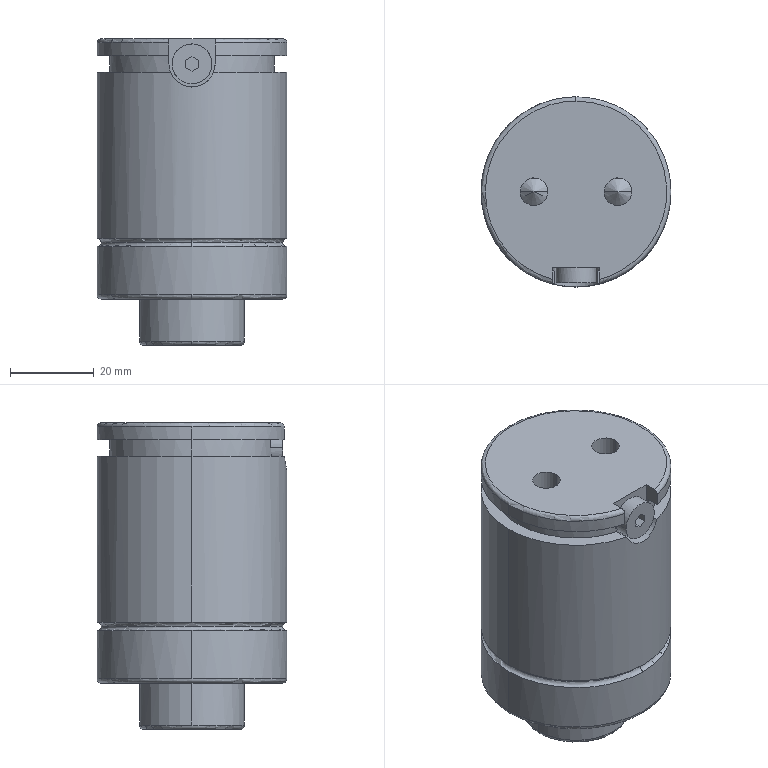Part | NX | features solid 2 | 1 solid | 55 faces | box 45.2 x 45.2 x 73 mm | volume 101993 mm3 | cylinder 21 | plane 16 | torus 10 | cone 8 | commonest cylinder face diameters 45.2 x7 6.6 x4 39.1 x3 4.9 x2 9.5 x2 25 x2